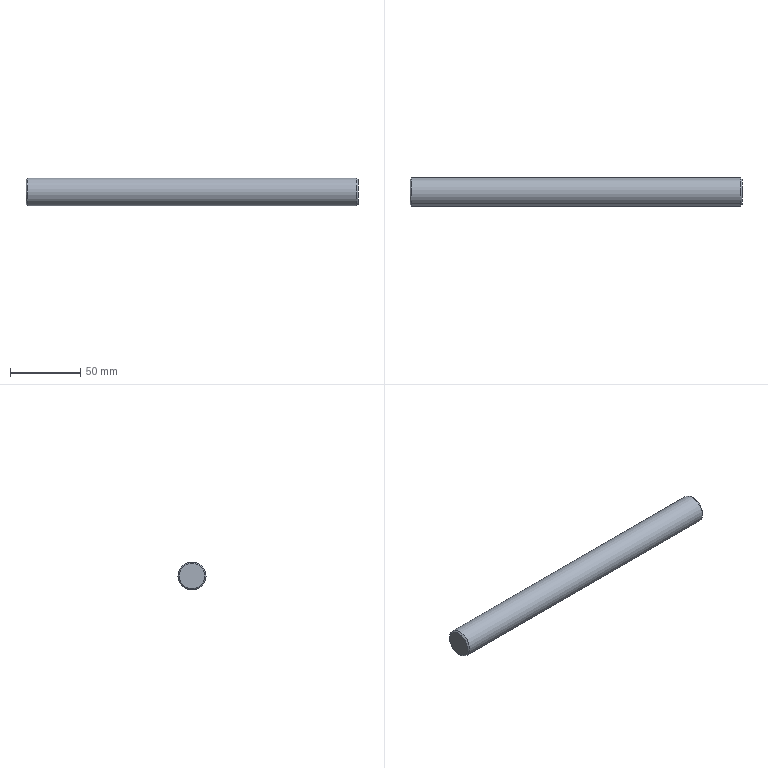Part | NX | features 000 2 | 1 solid | 5 faces | box 236 x 20 x 20 mm | volume 74081 mm3 | plane 2 | cone 2 | cylinder 1 | commonest cylinder face diameters 20 x1
STEP:
#1=CARTESIAN_POINT('',(-176.7,-269.8,-695.529));
#2=VERTEX_POINT('',#1);
#3=CARTESIAN_POINT('',(-176.7,-260.8,-695.529));
#4=DIRECTION('',(-1.,0.,0.));
#5=DIRECTION('',(0.,-1.,0.));
#6=AXIS2_PLACEMENT_3D('',#3,#4,#5);
#7=CIRCLE('',#6,9.);
#8=EDGE_CURVE('',#2,#2,#7,.T.);
#9=ORIENTED_EDGE('',*,*,#8,.T.);
#10=EDGE_LOOP('',(#9));
#11=FACE_BOUND('',#10,.T.);
#12=CARTESIAN_POINT('',(-176.7,-260.8,-695.529));
#13=DIRECTION('',(-1.,0.,0.));
#14=DIRECTION('',(0.,-1.,0.));
#15=AXIS2_PLACEMENT_3D('',#12,#13,#14);
#16=PLANE('',#15);
#17=ADVANCED_FACE('',(#11),#16,.T.);
#18=CARTESIAN_POINT('',(-175.7,-270.8,-695.529));
#19=VERTEX_POINT('',#18);
#20=CARTESIAN_POINT('',(-175.7,-260.8,-695.529));
#21=DIRECTION('',(-1.,0.,0.));
#22=DIRECTION('',(0.,-1.,0.));
#23=AXIS2_PLACEMENT_3D('',#20,#21,#22);
#24=CIRCLE('',#23,10.);
#25=EDGE_CURVE('',#19,#19,#24,.T.);
#26=ORIENTED_EDGE('',*,*,#25,.T.);
#27=EDGE_LOOP('',(#26));
#28=FACE_BOUND('',#27,.T.);
#29=ORIENTED_EDGE('',*,*,#8,.F.);
#30=EDGE_LOOP('',(#29));
#31=FACE_BOUND('',#30,.T.);
#32=CARTESIAN_POINT('',(-176.902,-260.8,-695.529));
#33=DIRECTION('',(1.,0.,0.));
#34=DIRECTION('',(0.,1.,0.));
#35=AXIS2_PLACEMENT_3D('',#32,#33,#34);
#36=CONICAL_SURFACE('',#35,8.798,0.7854);
#37=ADVANCED_FACE('',(#28,#31),#36,.T.);
#38=ORIENTED_EDGE('',*,*,#25,.F.);
#39=EDGE_LOOP('',(#38));
#40=FACE_BOUND('',#39,.T.);
#41=CARTESIAN_POINT('',(58.3,-270.8,-695.529));
#42=VERTEX_POINT('',#41);
#43=CARTESIAN_POINT('',(58.3,-260.8,-695.529));
#44=DIRECTION('',(1.,0.,0.));
#45=DIRECTION('',(0.,-1.,0.));
#46=AXIS2_PLACEMENT_3D('',#43,#44,#45);
#47=CIRCLE('',#46,10.);
#48=EDGE_CURVE('',#42,#42,#47,.T.);
#49=ORIENTED_EDGE('',*,*,#48,.F.);
#50=EDGE_LOOP('',(#49));
#51=FACE_BOUND('',#50,.T.);
#52=CARTESIAN_POINT('',(-176.7,-260.8,-695.529));
#53=DIRECTION('',(1.,0.,0.));
#54=DIRECTION('',(0.,1.,0.));
#55=AXIS2_PLACEMENT_3D('',#52,#53,#54);
#56=CYLINDRICAL_SURFACE('',#55,10.);
#57=ADVANCED_FACE('',(#40,#51),#56,.T.);
#58=CARTESIAN_POINT('',(59.3,-269.8,-695.529));
#59=VERTEX_POINT('',#58);
#60=CARTESIAN_POINT('',(59.3,-260.8,-695.529));
#61=DIRECTION('',(1.,0.,0.));
#62=DIRECTION('',(0.,-1.,0.));
#63=AXIS2_PLACEMENT_3D('',#60,#61,#62);
#64=CIRCLE('',#63,9.);
#65=EDGE_CURVE('',#59,#59,#64,.T.);
#66=ORIENTED_EDGE('',*,*,#65,.T.);
#67=EDGE_LOOP('',(#66));
#68=FACE_BOUND('',#67,.T.);
#69=CARTESIAN_POINT('',(59.3,-260.8,-695.529));
#70=DIRECTION('',(-1.,0.,0.));
#71=DIRECTION('',(0.,-1.,0.));
#72=AXIS2_PLACEMENT_3D('',#69,#70,#71);
#73=PLANE('',#72);
#74=ADVANCED_FACE('',(#68),#73,.F.);
#75=ORIENTED_EDGE('',*,*,#65,.F.);
#76=EDGE_LOOP('',(#75));
#77=FACE_BOUND('',#76,.T.);
#78=ORIENTED_EDGE('',*,*,#48,.T.);
#79=EDGE_LOOP('',(#78));
#80=FACE_BOUND('',#79,.T.);
#81=CARTESIAN_POINT('',(59.502,-260.8,-695.529));
#82=DIRECTION('',(-1.,0.,0.));
#83=DIRECTION('',(0.,-1.,0.));
#84=AXIS2_PLACEMENT_3D('',#81,#82,#83);
#85=CONICAL_SURFACE('',#84,8.798,0.7854);
#86=ADVANCED_FACE('',(#77,#80),#85,.T.);
#87=CLOSED_SHELL('',(#17,#37,#57,#74,#86));
#88=MANIFOLD_SOLID_BREP('',#87);
#89=(LENGTH_UNIT()NAMED_UNIT(*)SI_UNIT(.MILLI.,.METRE.));
#90=UNCERTAINTY_MEASURE_WITH_UNIT(LENGTH_MEASURE(0.00001),#89,'','');
#91=(NAMED_UNIT(*)PLANE_ANGLE_UNIT()SI_UNIT($,.RADIAN.));
#92=(NAMED_UNIT(*)SI_UNIT($,.STERADIAN.)SOLID_ANGLE_UNIT());
#93=(GEOMETRIC_REPRESENTATION_CONTEXT(3)GLOBAL_UNCERTAINTY_ASSIGNED_CONTEXT((#90))GLOBAL_UNIT_ASSIGNED_CONTEXT((#89,#91,#92))REPRESENTATION_CONTEXT('',''));
#94=ADVANCED_BREP_SHAPE_REPRESENTATION('',(#88),#93);